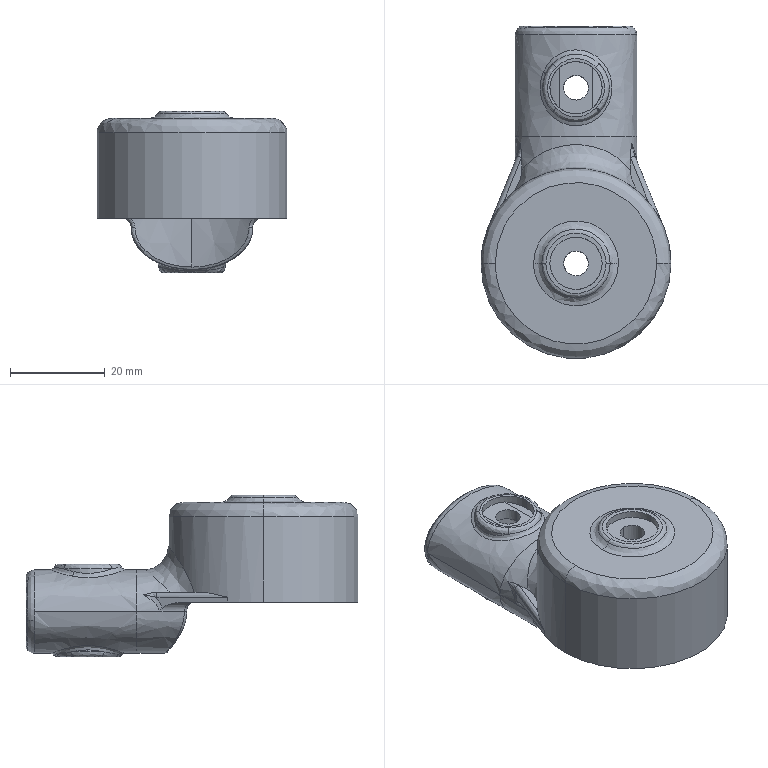Part | SolidWorks | features BaseBody 1 | 1 solid | 118 faces | box 40 x 70 x 34 mm | volume 17065 mm3 | spline 52 | cylinder 36 | plane 28 | cone 2 | commonest cylinder face diameters 5.2 x6 11 x6 14 x6 28.2 x5 2 x2 4 x2